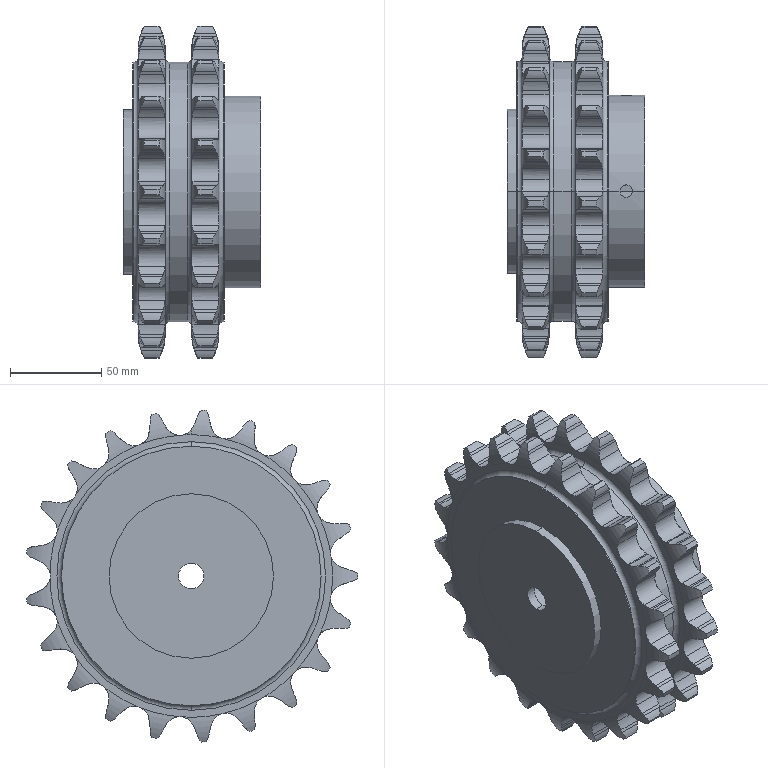Part | SolidWorks | features ICE 11, Chamfer 4, Revolution 3, Cut 2, CirPattern 1, DelFace 1, LPattern 1 | 2 solids | 491 faces | box 75 x 181.188 x 181.684 mm | volume 915452 mm3 | cylinder 293 | torus 96 | plane 96 | cone 6 | commonest cylinder face diameters 23.106 x90 41.467 x88 16.059 x54 182 x42 142 x6 6.8 x4